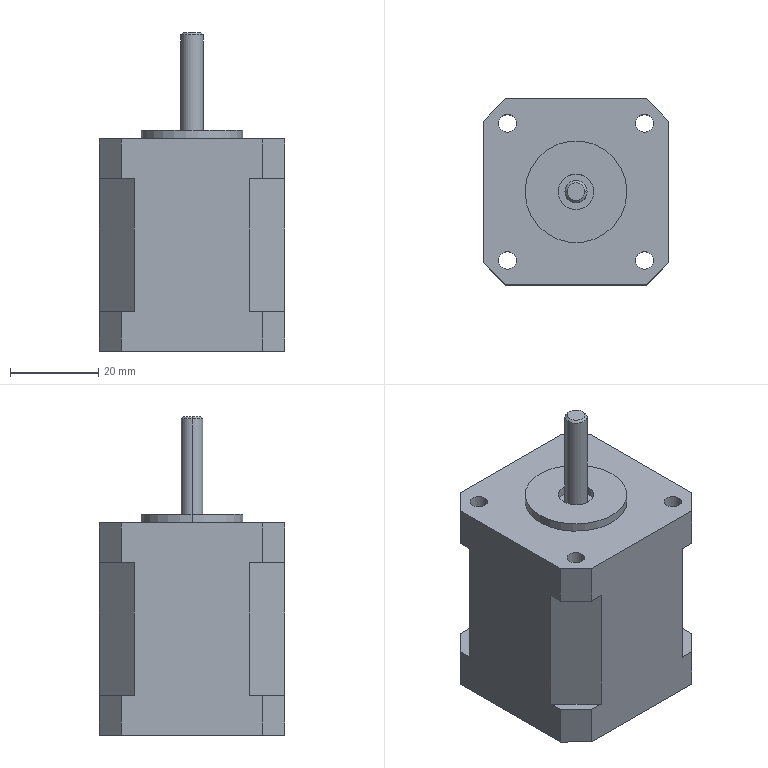Part | SolidWorks | features ICE 5, Chamfer 2, Extrusion 1, MirrorPattern 1 | 1 solid | 45 faces | box 42 x 42 x 72 mm | volume 78719 mm3 | plane 29 | cylinder 14 | cone 2 | commonest cylinder face diameters 4 x8 5 x2 8 x2 23 x2
STEP:
#1=CARTESIAN_POINT('',(-17.5,15.5,-24.));
#2=VERTEX_POINT('',#1);
#3=CARTESIAN_POINT('',(-13.5,15.5,-24.));
#4=VERTEX_POINT('',#3);
#5=CARTESIAN_POINT('',(-15.5,15.5,-24.));
#6=DIRECTION('',(0.,0.,1.));
#7=DIRECTION('',(1.,0.,0.));
#8=AXIS2_PLACEMENT_3D('',#5,#6,#7);
#9=CIRCLE('',#8,2.);
#10=EDGE_CURVE('',#2,#4,#9,.T.);
#11=ORIENTED_EDGE('',*,*,#10,.F.);
#12=CARTESIAN_POINT('',(-17.5,15.5,24.));
#13=VERTEX_POINT('',#12);
#14=CARTESIAN_POINT('',(-17.5,15.5,-24.));
#15=DIRECTION('',(0.,0.,1.));
#16=VECTOR('',#15,1000.);
#17=LINE('',#14,#16);
#18=EDGE_CURVE('',#2,#13,#17,.T.);
#19=ORIENTED_EDGE('',*,*,#18,.T.);
#20=CARTESIAN_POINT('',(-13.5,15.5,24.));
#21=VERTEX_POINT('',#20);
#22=CARTESIAN_POINT('',(-15.5,15.5,24.));
#23=DIRECTION('',(0.,0.,1.));
#24=DIRECTION('',(1.,0.,0.));
#25=AXIS2_PLACEMENT_3D('',#22,#23,#24);
#26=CIRCLE('',#25,2.);
#27=EDGE_CURVE('',#13,#21,#26,.T.);
#28=ORIENTED_EDGE('',*,*,#27,.T.);
#29=CARTESIAN_POINT('',(-13.5,15.5,-24.));
#30=DIRECTION('',(0.,0.,1.));
#31=VECTOR('',#30,1000.);
#32=LINE('',#29,#31);
#33=EDGE_CURVE('',#4,#21,#32,.T.);
#34=ORIENTED_EDGE('',*,*,#33,.F.);
#35=EDGE_LOOP('',(#11,#19,#28,#34));
#36=FACE_OUTER_BOUND('',#35,.T.);
#37=CARTESIAN_POINT('',(-15.5,15.5,-24.));
#38=DIRECTION('',(0.,0.,1.));
#39=DIRECTION('',(1.,0.,0.));
#40=AXIS2_PLACEMENT_3D('',#37,#38,#39);
#41=CYLINDRICAL_SURFACE('',#40,2.);
#42=ADVANCED_FACE('',(#36),#41,.F.);
#43=CARTESIAN_POINT('',(-17.5,-15.5,-24.));
#44=VERTEX_POINT('',#43);
#45=CARTESIAN_POINT('',(-13.5,-15.5,-24.));
#46=VERTEX_POINT('',#45);
#47=CARTESIAN_POINT('',(-15.5,-15.5,-24.));
#48=DIRECTION('',(0.,0.,1.));
#49=DIRECTION('',(1.,0.,0.));
#50=AXIS2_PLACEMENT_3D('',#47,#48,#49);
#51=CIRCLE('',#50,2.);
#52=EDGE_CURVE('',#44,#46,#51,.T.);
#53=ORIENTED_EDGE('',*,*,#52,.F.);
#54=CARTESIAN_POINT('',(-17.5,-15.5,24.));
#55=VERTEX_POINT('',#54);
#56=CARTESIAN_POINT('',(-17.5,-15.5,-24.));
#57=DIRECTION('',(0.,0.,1.));
#58=VECTOR('',#57,1000.);
#59=LINE('',#56,#58);
#60=EDGE_CURVE('',#44,#55,#59,.T.);
#61=ORIENTED_EDGE('',*,*,#60,.T.);
#62=CARTESIAN_POINT('',(-13.5,-15.5,24.));
#63=VERTEX_POINT('',#62);
#64=CARTESIAN_POINT('',(-15.5,-15.5,24.));
#65=DIRECTION('',(0.,0.,1.));
#66=DIRECTION('',(1.,0.,0.));
#67=AXIS2_PLACEMENT_3D('',#64,#65,#66);
#68=CIRCLE('',#67,2.);
#69=EDGE_CURVE('',#55,#63,#68,.T.);
#70=ORIENTED_EDGE('',*,*,#69,.T.);
#71=CARTESIAN_POINT('',(-13.5,-15.5,-24.));
#72=DIRECTION('',(0.,0.,1.));
#73=VECTOR('',#72,1000.);
#74=LINE('',#71,#73);
#75=EDGE_CURVE('',#46,#63,#74,.T.);
#76=ORIENTED_EDGE('',*,*,#75,.F.);
#77=EDGE_LOOP('',(#53,#61,#70,#76));
#78=FACE_OUTER_BOUND('',#77,.T.);
#79=CARTESIAN_POINT('',(-15.5,-15.5,-24.));
#80=DIRECTION('',(0.,0.,1.));
#81=DIRECTION('',(1.,0.,0.));
#82=AXIS2_PLACEMENT_3D('',#79,#80,#81);
#83=CYLINDRICAL_SURFACE('',#82,2.);
#84=ADVANCED_FACE('',(#78),#83,.F.);
#85=CARTESIAN_POINT('',(13.5,-15.5,-24.));
#86=VERTEX_POINT('',#85);
#87=CARTESIAN_POINT('',(17.5,-15.5,-24.));
#88=VERTEX_POINT('',#87);
#89=CARTESIAN_POINT('',(15.5,-15.5,-24.));
#90=DIRECTION('',(0.,0.,1.));
#91=DIRECTION('',(1.,0.,0.));
#92=AXIS2_PLACEMENT_3D('',#89,#90,#91);
#93=CIRCLE('',#92,2.);
#94=EDGE_CURVE('',#86,#88,#93,.T.);
#95=ORIENTED_EDGE('',*,*,#94,.F.);
#96=CARTESIAN_POINT('',(13.5,-15.5,24.));
#97=VERTEX_POINT('',#96);
#98=CARTESIAN_POINT('',(13.5,-15.5,-24.));
#99=DIRECTION('',(0.,0.,1.));
#100=VECTOR('',#99,1000.);
#101=LINE('',#98,#100);
#102=EDGE_CURVE('',#86,#97,#101,.T.);
#103=ORIENTED_EDGE('',*,*,#102,.T.);
#104=CARTESIAN_POINT('',(17.5,-15.5,24.));
#105=VERTEX_POINT('',#104);
#106=CARTESIAN_POINT('',(15.5,-15.5,24.));
#107=DIRECTION('',(0.,0.,1.));
#108=DIRECTION('',(1.,0.,0.));
#109=AXIS2_PLACEMENT_3D('',#106,#107,#108);
#110=CIRCLE('',#109,2.);
#111=EDGE_CURVE('',#97,#105,#110,.T.);
#112=ORIENTED_EDGE('',*,*,#111,.T.);
#113=CARTESIAN_POINT('',(17.5,-15.5,-24.));
#114=DIRECTION('',(0.,0.,1.));
#115=VECTOR('',#114,1000.);
#116=LINE('',#113,#115);
#117=EDGE_CURVE('',#88,#105,#116,.T.);
#118=ORIENTED_EDGE('',*,*,#117,.F.);
#119=EDGE_LOOP('',(#95,#103,#112,#118));
#120=FACE_OUTER_BOUND('',#119,.T.);
#121=CARTESIAN_POINT('',(15.5,-15.5,-24.));
#122=DIRECTION('',(0.,0.,1.));
#123=DIRECTION('',(1.,0.,0.));
#124=AXIS2_PLACEMENT_3D('',#121,#122,#123);
#125=CYLINDRICAL_SURFACE('',#124,2.);
#126=ADVANCED_FACE('',(#120),#125,.F.);
#127=CARTESIAN_POINT('',(13.5,15.5,-24.));
#128=VERTEX_POINT('',#127);
#129=CARTESIAN_POINT('',(17.5,15.5,-24.));
#130=VERTEX_POINT('',#129);
#131=CARTESIAN_POINT('',(15.5,15.5,-24.));
#132=DIRECTION('',(0.,0.,1.));
#133=DIRECTION('',(1.,0.,0.));
#134=AXIS2_PLACEMENT_3D('',#131,#132,#133);
#135=CIRCLE('',#134,2.);
#136=EDGE_CURVE('',#128,#130,#135,.T.);
#137=ORIENTED_EDGE('',*,*,#136,.F.);
#138=CARTESIAN_POINT('',(13.5,15.5,24.));
#139=VERTEX_POINT('',#138);
#140=CARTESIAN_POINT('',(13.5,15.5,-24.));
#141=DIRECTION('',(0.,0.,1.));
#142=VECTOR('',#141,1000.);
#143=LINE('',#140,#142);
#144=EDGE_CURVE('',#128,#139,#143,.T.);
#145=ORIENTED_EDGE('',*,*,#144,.T.);
#146=CARTESIAN_POINT('',(17.5,15.5,24.));
#147=VERTEX_POINT('',#146);
#148=CARTESIAN_POINT('',(15.5,15.5,24.));
#149=DIRECTION('',(0.,0.,1.));
#150=DIRECTION('',(1.,0.,0.));
#151=AXIS2_PLACEMENT_3D('',#148,#149,#150);
#152=CIRCLE('',#151,2.);
#153=EDGE_CURVE('',#139,#147,#152,.T.);
#154=ORIENTED_EDGE('',*,*,#153,.T.);
#155=CARTESIAN_POINT('',(17.5,15.5,-24.));
#156=DIRECTION('',(0.,0.,1.));
#157=VECTOR('',#156,1000.);
#158=LINE('',#155,#157);
#159=EDGE_CURVE('',#130,#147,#158,.T.);
#160=ORIENTED_EDGE('',*,*,#159,.F.);
#161=EDGE_LOOP('',(#137,#145,#154,#160));
#162=FACE_OUTER_BOUND('',#161,.T.);
#163=CARTESIAN_POINT('',(15.5,15.5,-24.));
#164=DIRECTION('',(0.,0.,1.));
#165=DIRECTION('',(1.,0.,0.));
#166=AXIS2_PLACEMENT_3D('',#163,#164,#165);
#167=CYLINDRICAL_SURFACE('',#166,2.);
#168=ADVANCED_FACE('',(#162),#167,.F.);
#169=CARTESIAN_POINT('',(2.,0.,48.));
#170=VERTEX_POINT('',#169);
#171=CARTESIAN_POINT('',(-2.,0.,48.));
#172=VERTEX_POINT('',#171);
#173=CARTESIAN_POINT('',(0.,0.,48.));
#174=DIRECTION('',(0.,0.,1.));
#175=DIRECTION('',(1.,0.,0.));
#176=AXIS2_PLACEMENT_3D('',#173,#174,#175);
#177=CIRCLE('',#176,2.);
#178=EDGE_CURVE('',#170,#172,#177,.T.);
#179=ORIENTED_EDGE('',*,*,#178,.F.);
#180=CARTESIAN_POINT('',(2.5,0.,47.5));
#181=VERTEX_POINT('',#180);
#182=CARTESIAN_POINT('',(2.,0.,48.));
#183=DIRECTION('',(0.7071,0.,-0.7071));
#184=VECTOR('',#183,1000.);
#185=LINE('',#182,#184);
#186=EDGE_CURVE('',#170,#181,#185,.T.);
#187=ORIENTED_EDGE('',*,*,#186,.T.);
#188=CARTESIAN_POINT('',(-2.5,0.,47.5));
#189=VERTEX_POINT('',#188);
#190=CARTESIAN_POINT('',(0.,0.,47.5));
#191=DIRECTION('',(0.,0.,-1.));
#192=DIRECTION('',(1.,0.,0.));
#193=AXIS2_PLACEMENT_3D('',#190,#191,#192);
#194=CIRCLE('',#193,2.5);
#195=EDGE_CURVE('',#189,#181,#194,.T.);
#196=ORIENTED_EDGE('',*,*,#195,.F.);
#197=CARTESIAN_POINT('',(-2.,0.,48.));
#198=DIRECTION('',(-0.7071,0.,-0.7071));
#199=VECTOR('',#198,1000.);
#200=LINE('',#197,#199);
#201=EDGE_CURVE('',#172,#189,#200,.T.);
#202=ORIENTED_EDGE('',*,*,#201,.F.);
#203=EDGE_LOOP('',(#179,#187,#196,#202));
#204=FACE_OUTER_BOUND('',#203,.T.);
#205=CARTESIAN_POINT('',(0.,0.,48.));
#206=DIRECTION('',(0.,0.,-1.));
#207=DIRECTION('',(-1.,0.,0.));
#208=AXIS2_PLACEMENT_3D('',#205,#206,#207);
#209=CONICAL_SURFACE('',#208,2.,0.7854);
#210=ADVANCED_FACE('',(#204),#209,.T.);
#211=ORIENTED_EDGE('',*,*,#195,.T.);
#212=CARTESIAN_POINT('',(2.5,0.,24.));
#213=VERTEX_POINT('',#212);
#214=CARTESIAN_POINT('',(2.5,0.,48.));
#215=DIRECTION('',(0.,0.,-1.));
#216=VECTOR('',#215,1000.);
#217=LINE('',#214,#216);
#218=EDGE_CURVE('',#181,#213,#217,.T.);
#219=ORIENTED_EDGE('',*,*,#218,.T.);
#220=CARTESIAN_POINT('',(-2.5,0.,24.));
#221=VERTEX_POINT('',#220);
#222=CARTESIAN_POINT('',(0.,0.,24.));
#223=DIRECTION('',(0.,0.,1.));
#224=DIRECTION('',(1.,0.,0.));
#225=AXIS2_PLACEMENT_3D('',#222,#223,#224);
#226=CIRCLE('',#225,2.5);
#227=EDGE_CURVE('',#213,#221,#226,.T.);
#228=ORIENTED_EDGE('',*,*,#227,.T.);
#229=CARTESIAN_POINT('',(-2.5,0.,48.));
#230=DIRECTION('',(0.,0.,-1.));
#231=VECTOR('',#230,1000.);
#232=LINE('',#229,#231);
#233=EDGE_CURVE('',#189,#221,#232,.T.);
#234=ORIENTED_EDGE('',*,*,#233,.F.);
#235=EDGE_LOOP('',(#211,#219,#228,#234));
#236=FACE_OUTER_BOUND('',#235,.T.);
#237=CARTESIAN_POINT('',(0.,0.,48.));
#238=DIRECTION('',(0.,0.,-1.));
#239=DIRECTION('',(-1.,0.,0.));
#240=AXIS2_PLACEMENT_3D('',#237,#238,#239);
#241=CYLINDRICAL_SURFACE('',#240,2.5);
#242=ADVANCED_FACE('',(#236),#241,.T.);
#243=CARTESIAN_POINT('',(-4.,0.,24.));
#244=VERTEX_POINT('',#243);
#245=CARTESIAN_POINT('',(4.,0.,24.));
#246=VERTEX_POINT('',#245);
#247=CARTESIAN_POINT('',(0.,0.,24.));
#248=DIRECTION('',(0.,0.,1.));
#249=DIRECTION('',(1.,0.,0.));
#250=AXIS2_PLACEMENT_3D('',#247,#248,#249);
#251=CIRCLE('',#250,4.);
#252=EDGE_CURVE('',#244,#246,#251,.T.);
#253=ORIENTED_EDGE('',*,*,#252,.F.);
#254=CARTESIAN_POINT('',(-4.,0.,26.));
#255=VERTEX_POINT('',#254);
#256=CARTESIAN_POINT('',(-4.,0.,24.));
#257=DIRECTION('',(0.,0.,1.));
#258=VECTOR('',#257,1000.);
#259=LINE('',#256,#258);
#260=EDGE_CURVE('',#244,#255,#259,.T.);
#261=ORIENTED_EDGE('',*,*,#260,.T.);
#262=CARTESIAN_POINT('',(4.,0.,26.));
#263=VERTEX_POINT('',#262);
#264=CARTESIAN_POINT('',(0.,0.,26.));
#265=DIRECTION('',(0.,0.,1.));
#266=DIRECTION('',(1.,0.,0.));
#267=AXIS2_PLACEMENT_3D('',#264,#265,#266);
#268=CIRCLE('',#267,4.);
#269=EDGE_CURVE('',#255,#263,#268,.T.);
#270=ORIENTED_EDGE('',*,*,#269,.T.);
#271=CARTESIAN_POINT('',(4.,0.,24.));
#272=DIRECTION('',(0.,0.,1.));
#273=VECTOR('',#272,1000.);
#274=LINE('',#271,#273);
#275=EDGE_CURVE('',#246,#263,#274,.T.);
#276=ORIENTED_EDGE('',*,*,#275,.F.);
#277=EDGE_LOOP('',(#253,#261,#270,#276));
#278=FACE_OUTER_BOUND('',#277,.T.);
#279=CARTESIAN_POINT('',(0.,0.,24.));
#280=DIRECTION('',(0.,0.,1.));
#281=DIRECTION('',(1.,0.,0.));
#282=AXIS2_PLACEMENT_3D('',#279,#280,#281);
#283=CYLINDRICAL_SURFACE('',#282,4.);
#284=ADVANCED_FACE('',(#278),#283,.F.);
#285=CARTESIAN_POINT('',(11.5,0.,26.));
#286=VERTEX_POINT('',#285);
#287=CARTESIAN_POINT('',(-11.5,0.,26.));
#288=VERTEX_POINT('',#287);
#289=CARTESIAN_POINT('',(0.,0.,26.));
#290=DIRECTION('',(0.,0.,1.));
#291=DIRECTION('',(1.,0.,0.));
#292=AXIS2_PLACEMENT_3D('',#289,#290,#291);
#293=CIRCLE('',#292,11.5);
#294=EDGE_CURVE('',#286,#288,#293,.T.);
#295=ORIENTED_EDGE('',*,*,#294,.F.);
#296=CARTESIAN_POINT('',(11.5,0.,24.));
#297=VERTEX_POINT('',#296);
#298=CARTESIAN_POINT('',(11.5,0.,26.));
#299=DIRECTION('',(0.,0.,-1.));
#300=VECTOR('',#299,1000.);
#301=LINE('',#298,#300);
#302=EDGE_CURVE('',#286,#297,#301,.T.);
#303=ORIENTED_EDGE('',*,*,#302,.T.);
#304=CARTESIAN_POINT('',(-11.5,0.,24.));
#305=VERTEX_POINT('',#304);
#306=CARTESIAN_POINT('',(0.,0.,24.));
#307=DIRECTION('',(0.,0.,1.));
#308=DIRECTION('',(-1.,0.,0.));
#309=AXIS2_PLACEMENT_3D('',#306,#307,#308);
#310=CIRCLE('',#309,11.5);
#311=EDGE_CURVE('',#297,#305,#310,.T.);
#312=ORIENTED_EDGE('',*,*,#311,.T.);
#313=CARTESIAN_POINT('',(-11.5,0.,26.));
#314=DIRECTION('',(0.,0.,-1.));
#315=VECTOR('',#314,1000.);
#316=LINE('',#313,#315);
#317=EDGE_CURVE('',#288,#305,#316,.T.);
#318=ORIENTED_EDGE('',*,*,#317,.F.);
#319=EDGE_LOOP('',(#295,#303,#312,#318));
#320=FACE_OUTER_BOUND('',#319,.T.);
#321=CARTESIAN_POINT('',(0.,0.,26.));
#322=DIRECTION('',(0.,0.,-1.));
#323=DIRECTION('',(-1.,0.,0.));
#324=AXIS2_PLACEMENT_3D('',#321,#322,#323);
#325=CYLINDRICAL_SURFACE('',#324,11.5);
#326=ADVANCED_FACE('',(#320),#325,.T.);
#327=CARTESIAN_POINT('',(0.,0.,26.));
#328=DIRECTION('',(0.,0.,1.));
#329=DIRECTION('',(1.,0.,0.));
#330=AXIS2_PLACEMENT_3D('',#327,#328,#329);
#331=CIRCLE('',#330,4.);
#332=EDGE_CURVE('',#263,#255,#331,.T.);
#333=ORIENTED_EDGE('',*,*,#332,.F.);
#334=ORIENTED_EDGE('',*,*,#269,.F.);
#335=EDGE_LOOP('',(#333,#334));
#336=FACE_BOUND('',#335,.T.);
#337=CARTESIAN_POINT('',(0.,0.,26.));
#338=DIRECTION('',(0.,0.,1.));
#339=DIRECTION('',(1.,0.,0.));
#340=AXIS2_PLACEMENT_3D('',#337,#338,#339);
#341=CIRCLE('',#340,11.5);
#342=EDGE_CURVE('',#288,#286,#341,.T.);
#343=ORIENTED_EDGE('',*,*,#342,.T.);
#344=ORIENTED_EDGE('',*,*,#294,.T.);
#345=EDGE_LOOP('',(#343,#344));
#346=FACE_OUTER_BOUND('',#345,.T.);
#347=CARTESIAN_POINT('',(0.,0.,26.));
#348=DIRECTION('',(0.,0.,1.));
#349=DIRECTION('',(1.,0.,0.));
#350=AXIS2_PLACEMENT_3D('',#347,#348,#349);
#351=PLANE('',#350);
#352=ADVANCED_FACE('',(#336,#346),#351,.T.);
#353=CARTESIAN_POINT('',(-15.5,15.5,24.));
#354=DIRECTION('',(0.,0.,1.));
#355=DIRECTION('',(1.,0.,0.));
#356=AXIS2_PLACEMENT_3D('',#353,#354,#355);
#357=CIRCLE('',#356,2.);
#358=EDGE_CURVE('',#21,#13,#357,.T.);
#359=ORIENTED_EDGE('',*,*,#358,.F.);
#360=ORIENTED_EDGE('',*,*,#27,.F.);
#361=EDGE_LOOP('',(#359,#360));
#362=FACE_BOUND('',#361,.T.);
#363=CARTESIAN_POINT('',(-15.5,-15.5,24.));
#364=DIRECTION('',(0.,0.,1.));
#365=DIRECTION('',(1.,0.,0.));
#366=AXIS2_PLACEMENT_3D('',#363,#364,#365);
#367=CIRCLE('',#366,2.);
#368=EDGE_CURVE('',#63,#55,#367,.T.);
#369=ORIENTED_EDGE('',*,*,#368,.F.);
#370=ORIENTED_EDGE('',*,*,#69,.F.);
#371=EDGE_LOOP('',(#369,#370));
#372=FACE_BOUND('',#371,.T.);
#373=CARTESIAN_POINT('',(15.5,-15.5,24.));
#374=DIRECTION('',(0.,0.,1.));
#375=DIRECTION('',(1.,0.,0.));
#376=AXIS2_PLACEMENT_3D('',#373,#374,#375);
#377=CIRCLE('',#376,2.);
#378=EDGE_CURVE('',#105,#97,#377,.T.);
#379=ORIENTED_EDGE('',*,*,#378,.F.);
#380=ORIENTED_EDGE('',*,*,#111,.F.);
#381=EDGE_LOOP('',(#379,#380));
#382=FACE_BOUND('',#381,.T.);
#383=CARTESIAN_POINT('',(15.5,15.5,24.));
#384=DIRECTION('',(0.,0.,1.));
#385=DIRECTION('',(1.,0.,0.));
#386=AXIS2_PLACEMENT_3D('',#383,#384,#385);
#387=CIRCLE('',#386,2.);
#388=EDGE_CURVE('',#147,#139,#387,.T.);
#389=ORIENTED_EDGE('',*,*,#388,.F.);
#390=ORIENTED_EDGE('',*,*,#153,.F.);
#391=EDGE_LOOP('',(#389,#390));
#392=FACE_BOUND('',#391,.T.);
#393=CARTESIAN_POINT('',(-16.,21.,24.));
#394=VERTEX_POINT('',#393);
#395=CARTESIAN_POINT('',(-21.,16.,24.));
#396=VERTEX_POINT('',#395);
#397=CARTESIAN_POINT('',(-16.,21.,24.));
#398=DIRECTION('',(-0.7071,-0.7071,0.));
#399=VECTOR('',#398,1000.);
#400=LINE('',#397,#399);
#401=EDGE_CURVE('',#394,#396,#400,.T.);
#402=ORIENTED_EDGE('',*,*,#401,.T.);
#403=CARTESIAN_POINT('',(-21.,-16.,24.));
#404=VERTEX_POINT('',#403);
#405=CARTESIAN_POINT('',(-21.,-16.,24.));
#406=DIRECTION('',(0.,-1.,0.));
#407=VECTOR('',#406,1000.);
#408=LINE('',#405,#407);
#409=EDGE_CURVE('',#396,#404,#408,.T.);
#410=ORIENTED_EDGE('',*,*,#409,.T.);
#411=CARTESIAN_POINT('',(-16.,-21.,24.));
#412=VERTEX_POINT('',#411);
#413=CARTESIAN_POINT('',(-16.,-21.,24.));
#414=DIRECTION('',(0.7071,-0.7071,0.));
#415=VECTOR('',#414,1000.);
#416=LINE('',#413,#415);
#417=EDGE_CURVE('',#404,#412,#416,.T.);
#418=ORIENTED_EDGE('',*,*,#417,.T.);
#419=CARTESIAN_POINT('',(16.,-21.,24.));
#420=VERTEX_POINT('',#419);
#421=CARTESIAN_POINT('',(16.,-21.,24.));
#422=DIRECTION('',(1.,0.,0.));
#423=VECTOR('',#422,1000.);
#424=LINE('',#421,#423);
#425=EDGE_CURVE('',#412,#420,#424,.T.);
#426=ORIENTED_EDGE('',*,*,#425,.T.);
#427=CARTESIAN_POINT('',(21.,-16.,24.));
#428=VERTEX_POINT('',#427);
#429=CARTESIAN_POINT('',(21.,-16.,24.));
#430=DIRECTION('',(0.7071,0.7071,0.));
#431=VECTOR('',#430,1000.);
#432=LINE('',#429,#431);
#433=EDGE_CURVE('',#420,#428,#432,.T.);
#434=ORIENTED_EDGE('',*,*,#433,.T.);
#435=CARTESIAN_POINT('',(21.,16.,24.));
#436=VERTEX_POINT('',#435);
#437=CARTESIAN_POINT('',(21.,-16.,24.));
#438=DIRECTION('',(0.,1.,0.));
#439=VECTOR('',#438,1000.);
#440=LINE('',#437,#439);
#441=EDGE_CURVE('',#428,#436,#440,.T.);
#442=ORIENTED_EDGE('',*,*,#441,.T.);
#443=CARTESIAN_POINT('',(16.,21.,24.));
#444=VERTEX_POINT('',#443);
#445=CARTESIAN_POINT('',(21.,16.,24.));
#446=DIRECTION('',(-0.7071,0.7071,0.));
#447=VECTOR('',#446,1000.);
#448=LINE('',#445,#447);
#449=EDGE_CURVE('',#436,#444,#448,.T.);
#450=ORIENTED_EDGE('',*,*,#449,.T.);
#451=CARTESIAN_POINT('',(16.,21.,24.));
#452=DIRECTION('',(-1.,0.,0.));
#453=VECTOR('',#452,1000.);
#454=LINE('',#451,#453);
#455=EDGE_CURVE('',#444,#394,#454,.T.);
#456=ORIENTED_EDGE('',*,*,#455,.T.);
#457=EDGE_LOOP('',(#402,#410,#418,#426,#434,#442,#450,#456));
#458=FACE_OUTER_BOUND('',#457,.T.);
#459=CARTESIAN_POINT('',(0.,0.,24.));
#460=DIRECTION('',(0.,0.,1.));
#461=DIRECTION('',(-1.,0.,0.));
#462=AXIS2_PLACEMENT_3D('',#459,#460,#461);
#463=CIRCLE('',#462,11.5);
#464=EDGE_CURVE('',#305,#297,#463,.T.);
#465=ORIENTED_EDGE('',*,*,#464,.F.);
#466=ORIENTED_EDGE('',*,*,#311,.F.);
#467=EDGE_LOOP('',(#465,#466));
#468=FACE_BOUND('',#467,.T.);
#469=CARTESIAN_POINT('',(0.,0.,24.));
#470=DIRECTION('',(0.,0.,-1.));
#471=DIRECTION('',(-1.,0.,0.));
#472=AXIS2_PLACEMENT_3D('',#469,#470,#471);
#473=PLANE('',#472);
#474=ADVANCED_FACE('',(#362,#372,#382,#392,#458,#468),#473,.F.);
#475=CARTESIAN_POINT('',(-21.,13.,15.));
#476=VERTEX_POINT('',#475);
#477=CARTESIAN_POINT('',(-21.,13.,-15.));
#478=VERTEX_POINT('',#477);
#479=CARTESIAN_POINT('',(-21.,13.,15.));
#480=DIRECTION('',(0.,0.,-1.));
#481=VECTOR('',#480,1000.);
#482=LINE('',#479,#481);
#483=EDGE_CURVE('',#476,#478,#482,.T.);
#484=ORIENTED_EDGE('',*,*,#483,.T.);
#485=CARTESIAN_POINT('',(-21.,16.,-15.));
#486=VERTEX_POINT('',#485);
#487=CARTESIAN_POINT('',(-21.,-16.,-15.));
#488=DIRECTION('',(0.,-1.,0.));
#489=VECTOR('',#488,1000.);
#490=LINE('',#487,#489);
#491=EDGE_CURVE('',#486,#478,#490,.T.);
#492=ORIENTED_EDGE('',*,*,#491,.F.);
#493=CARTESIAN_POINT('',(-21.,16.,-24.));
#494=VERTEX_POINT('',#493);
#495=CARTESIAN_POINT('',(-21.,16.,-24.));
#496=DIRECTION('',(0.,0.,1.));
#497=VECTOR('',#496,1000.);
#498=LINE('',#495,#497);
#499=EDGE_CURVE('',#494,#486,#498,.T.);
#500=ORIENTED_EDGE('',*,*,#499,.F.);
#501=CARTESIAN_POINT('',(-21.,-16.,-24.));
#502=VERTEX_POINT('',#501);
#503=CARTESIAN_POINT('',(-21.,-16.,-24.));
#504=DIRECTION('',(0.,-1.,0.));
#505=VECTOR('',#504,1000.);
#506=LINE('',#503,#505);
#507=EDGE_CURVE('',#494,#502,#506,.T.);
#508=ORIENTED_EDGE('',*,*,#507,.T.);
#509=CARTESIAN_POINT('',(-21.,-16.,-15.));
#510=VERTEX_POINT('',#509);
#511=CARTESIAN_POINT('',(-21.,-16.,-24.));
#512=DIRECTION('',(0.,0.,1.));
#513=VECTOR('',#512,1000.);
#514=LINE('',#511,#513);
#515=EDGE_CURVE('',#502,#510,#514,.T.);
#516=ORIENTED_EDGE('',*,*,#515,.T.);
#517=CARTESIAN_POINT('',(-21.,-13.,-15.));
#518=VERTEX_POINT('',#517);
#519=CARTESIAN_POINT('',(-21.,-16.,-15.));
#520=DIRECTION('',(0.,-1.,0.));
#521=VECTOR('',#520,1000.);
#522=LINE('',#519,#521);
#523=EDGE_CURVE('',#518,#510,#522,.T.);
#524=ORIENTED_EDGE('',*,*,#523,.F.);
#525=CARTESIAN_POINT('',(-21.,-13.,15.));
#526=VERTEX_POINT('',#525);
#527=CARTESIAN_POINT('',(-21.,-13.,15.));
#528=DIRECTION('',(0.,0.,1.));
#529=VECTOR('',#528,1000.);
#530=LINE('',#527,#529);
#531=EDGE_CURVE('',#518,#526,#530,.T.);
#532=ORIENTED_EDGE('',*,*,#531,.T.);
#533=CARTESIAN_POINT('',(-21.,-16.,15.));
#534=VERTEX_POINT('',#533);
#535=CARTESIAN_POINT('',(-21.,-16.,15.));
#536=DIRECTION('',(0.,-1.,0.));
#537=VECTOR('',#536,1000.);
#538=LINE('',#535,#537);
#539=EDGE_CURVE('',#526,#534,#538,.T.);
#540=ORIENTED_EDGE('',*,*,#539,.T.);
#541=CARTESIAN_POINT('',(-21.,-16.,24.));
#542=DIRECTION('',(0.,0.,-1.));
#543=VECTOR('',#542,1000.);
#544=LINE('',#541,#543);
#545=EDGE_CURVE('',#404,#534,#544,.T.);
#546=ORIENTED_EDGE('',*,*,#545,.F.);
#547=ORIENTED_EDGE('',*,*,#409,.F.);
#548=CARTESIAN_POINT('',(-21.,16.,15.));
#549=VERTEX_POINT('',#548);
#550=CARTESIAN_POINT('',(-21.,16.,24.));
#551=DIRECTION('',(0.,0.,-1.));
#552=VECTOR('',#551,1000.);
#553=LINE('',#550,#552);
#554=EDGE_CURVE('',#396,#549,#553,.T.);
#555=ORIENTED_EDGE('',*,*,#554,.T.);
#556=CARTESIAN_POINT('',(-21.,-16.,15.));
#557=DIRECTION('',(0.,-1.,0.));
#558=VECTOR('',#557,1000.);
#559=LINE('',#556,#558);
#560=EDGE_CURVE('',#549,#476,#559,.T.);
#561=ORIENTED_EDGE('',*,*,#560,.T.);
#562=EDGE_LOOP('',(#484,#492,#500,#508,#516,#524,#532,#540,#546,#547,#555,#561));
#563=FACE_OUTER_BOUND('',#562,.T.);
#564=CARTESIAN_POINT('',(-21.,-21.,15.));
#565=DIRECTION('',(1.,0.,0.));
#566=DIRECTION('',(0.,0.,-1.));
#567=AXIS2_PLACEMENT_3D('',#564,#565,#566);
#568=PLANE('',#567);
#569=ADVANCED_FACE('',(#563),#568,.F.);
#570=CARTESIAN_POINT('',(13.,-21.,-15.));
#571=VERTEX_POINT('',#570);
#572=CARTESIAN_POINT('',(13.,-21.,15.));
#573=VERTEX_POINT('',#572);
#574=CARTESIAN_POINT('',(13.,-21.,15.));
#575=DIRECTION('',(0.,0.,1.));
#576=VECTOR('',#575,1000.);
#577=LINE('',#574,#576);
#578=EDGE_CURVE('',#571,#573,#577,.T.);
#579=ORIENTED_EDGE('',*,*,#578,.T.);
#580=CARTESIAN_POINT('',(16.,-21.,15.));
#581=VERTEX_POINT('',#580);
#582=CARTESIAN_POINT('',(16.,-21.,15.));
#583=DIRECTION('',(1.,0.,0.));
#584=VECTOR('',#583,1000.);
#585=LINE('',#582,#584);
#586=EDGE_CURVE('',#573,#581,#585,.T.);
#587=ORIENTED_EDGE('',*,*,#586,.T.);
#588=CARTESIAN_POINT('',(16.,-21.,24.));
#589=DIRECTION('',(0.,0.,-1.));
#590=VECTOR('',#589,1000.);
#591=LINE('',#588,#590);
#592=EDGE_CURVE('',#420,#581,#591,.T.);
#593=ORIENTED_EDGE('',*,*,#592,.F.);
#594=ORIENTED_EDGE('',*,*,#425,.F.);
#595=CARTESIAN_POINT('',(-16.,-21.,15.));
#596=VERTEX_POINT('',#595);
#597=CARTESIAN_POINT('',(-16.,-21.,24.));
#598=DIRECTION('',(0.,0.,-1.));
#599=VECTOR('',#598,1000.);
#600=LINE('',#597,#599);
#601=EDGE_CURVE('',#412,#596,#600,.T.);
#602=ORIENTED_EDGE('',*,*,#601,.T.);
#603=CARTESIAN_POINT('',(-13.,-21.,15.));
#604=VERTEX_POINT('',#603);
#605=CARTESIAN_POINT('',(16.,-21.,15.));
#606=DIRECTION('',(1.,0.,0.));
#607=VECTOR('',#606,1000.);
#608=LINE('',#605,#607);
#609=EDGE_CURVE('',#596,#604,#608,.T.);
#610=ORIENTED_EDGE('',*,*,#609,.T.);
#611=CARTESIAN_POINT('',(-13.,-21.,-15.));
#612=VERTEX_POINT('',#611);
#613=CARTESIAN_POINT('',(-13.,-21.,15.));
#614=DIRECTION('',(0.,0.,-1.));
#615=VECTOR('',#614,1000.);
#616=LINE('',#613,#615);
#617=EDGE_CURVE('',#604,#612,#616,.T.);
#618=ORIENTED_EDGE('',*,*,#617,.T.);
#619=CARTESIAN_POINT('',(-16.,-21.,-15.));
#620=VERTEX_POINT('',#619);
#621=CARTESIAN_POINT('',(16.,-21.,-15.));
#622=DIRECTION('',(1.,0.,0.));
#623=VECTOR('',#622,1000.);
#624=LINE('',#621,#623);
#625=EDGE_CURVE('',#620,#612,#624,.T.);
#626=ORIENTED_EDGE('',*,*,#625,.F.);
#627=CARTESIAN_POINT('',(-16.,-21.,-24.));
#628=VERTEX_POINT('',#627);
#629=CARTESIAN_POINT('',(-16.,-21.,-24.));
#630=DIRECTION('',(0.,0.,1.));
#631=VECTOR('',#630,1000.);
#632=LINE('',#629,#631);
#633=EDGE_CURVE('',#628,#620,#632,.T.);
#634=ORIENTED_EDGE('',*,*,#633,.F.);
#635=CARTESIAN_POINT('',(16.,-21.,-24.));
#636=VERTEX_POINT('',#635);
#637=CARTESIAN_POINT('',(16.,-21.,-24.));
#638=DIRECTION('',(1.,0.,0.));
#639=VECTOR('',#638,1000.);
#640=LINE('',#637,#639);
#641=EDGE_CURVE('',#628,#636,#640,.T.);
#642=ORIENTED_EDGE('',*,*,#641,.T.);
#643=CARTESIAN_POINT('',(16.,-21.,-15.));
#644=VERTEX_POINT('',#643);
#645=CARTESIAN_POINT('',(16.,-21.,-24.));
#646=DIRECTION('',(0.,0.,1.));
#647=VECTOR('',#646,1000.);
#648=LINE('',#645,#647);
#649=EDGE_CURVE('',#636,#644,#648,.T.);
#650=ORIENTED_EDGE('',*,*,#649,.T.);
#651=CARTESIAN_POINT('',(16.,-21.,-15.));
#652=DIRECTION('',(1.,0.,0.));
#653=VECTOR('',#652,1000.);
#654=LINE('',#651,#653);
#655=EDGE_CURVE('',#571,#644,#654,.T.);
#656=ORIENTED_EDGE('',*,*,#655,.F.);
#657=EDGE_LOOP('',(#579,#587,#593,#594,#602,#610,#618,#626,#634,#642,#650,#656));
#658=FACE_OUTER_BOUND('',#657,.T.);
#659=CARTESIAN_POINT('',(21.,-21.,15.));
#660=DIRECTION('',(0.,1.,0.));
#661=DIRECTION('',(-1.,0.,0.));
#662=AXIS2_PLACEMENT_3D('',#659,#660,#661);
#663=PLANE('',#662);
#664=ADVANCED_FACE('',(#658),#663,.F.);
#665=CARTESIAN_POINT('',(21.,13.,-15.));
#666=VERTEX_POINT('',#665);
#667=CARTESIAN_POINT('',(21.,13.,15.));
#668=VERTEX_POINT('',#667);
#669=CARTESIAN_POINT('',(21.,13.,15.));
#670=DIRECTION('',(0.,0.,1.));
#671=VECTOR('',#670,1000.);
#672=LINE('',#669,#671);
#673=EDGE_CURVE('',#666,#668,#672,.T.);
#674=ORIENTED_EDGE('',*,*,#673,.T.);
#675=CARTESIAN_POINT('',(21.,16.,15.));
#676=VERTEX_POINT('',#675);
#677=CARTESIAN_POINT('',(21.,-16.,15.));
#678=DIRECTION('',(0.,1.,0.));
#679=VECTOR('',#678,1000.);
#680=LINE('',#677,#679);
#681=EDGE_CURVE('',#668,#676,#680,.T.);
#682=ORIENTED_EDGE('',*,*,#681,.T.);
#683=CARTESIAN_POINT('',(21.,16.,24.));
#684=DIRECTION('',(0.,0.,-1.));
#685=VECTOR('',#684,1000.);
#686=LINE('',#683,#685);
#687=EDGE_CURVE('',#436,#676,#686,.T.);
#688=ORIENTED_EDGE('',*,*,#687,.F.);
#689=ORIENTED_EDGE('',*,*,#441,.F.);
#690=CARTESIAN_POINT('',(21.,-16.,15.));
#691=VERTEX_POINT('',#690);
#692=CARTESIAN_POINT('',(21.,-16.,24.));
#693=DIRECTION('',(0.,0.,-1.));
#694=VECTOR('',#693,1000.);
#695=LINE('',#692,#694);
#696=EDGE_CURVE('',#428,#691,#695,.T.);
#697=ORIENTED_EDGE('',*,*,#696,.T.);
#698=CARTESIAN_POINT('',(21.,-13.,15.));
#699=VERTEX_POINT('',#698);
#700=CARTESIAN_POINT('',(21.,-16.,15.));
#701=DIRECTION('',(0.,1.,0.));
#702=VECTOR('',#701,1000.);
#703=LINE('',#700,#702);
#704=EDGE_CURVE('',#691,#699,#703,.T.);
#705=ORIENTED_EDGE('',*,*,#704,.T.);
#706=CARTESIAN_POINT('',(21.,-13.,-15.));
#707=VERTEX_POINT('',#706);
#708=CARTESIAN_POINT('',(21.,-13.,15.));
#709=DIRECTION('',(0.,0.,-1.));
#710=VECTOR('',#709,1000.);
#711=LINE('',#708,#710);
#712=EDGE_CURVE('',#699,#707,#711,.T.);
#713=ORIENTED_EDGE('',*,*,#712,.T.);
#714=CARTESIAN_POINT('',(21.,-16.,-15.));
#715=VERTEX_POINT('',#714);
#716=CARTESIAN_POINT('',(21.,-16.,-15.));
#717=DIRECTION('',(0.,1.,0.));
#718=VECTOR('',#717,1000.);
#719=LINE('',#716,#718);
#720=EDGE_CURVE('',#715,#707,#719,.T.);
#721=ORIENTED_EDGE('',*,*,#720,.F.);
#722=CARTESIAN_POINT('',(21.,-16.,-24.));
#723=VERTEX_POINT('',#722);
#724=CARTESIAN_POINT('',(21.,-16.,-24.));
#725=DIRECTION('',(0.,0.,1.));
#726=VECTOR('',#725,1000.);
#727=LINE('',#724,#726);
#728=EDGE_CURVE('',#723,#715,#727,.T.);
#729=ORIENTED_EDGE('',*,*,#728,.F.);
#730=CARTESIAN_POINT('',(21.,16.,-24.));
#731=VERTEX_POINT('',#730);
#732=CARTESIAN_POINT('',(21.,-16.,-24.));
#733=DIRECTION('',(0.,1.,0.));
#734=VECTOR('',#733,1000.);
#735=LINE('',#732,#734);
#736=EDGE_CURVE('',#723,#731,#735,.T.);
#737=ORIENTED_EDGE('',*,*,#736,.T.);
#738=CARTESIAN_POINT('',(21.,16.,-15.));
#739=VERTEX_POINT('',#738);
#740=CARTESIAN_POINT('',(21.,16.,-24.));
#741=DIRECTION('',(0.,0.,1.));
#742=VECTOR('',#741,1000.);
#743=LINE('',#740,#742);
#744=EDGE_CURVE('',#731,#739,#743,.T.);
#745=ORIENTED_EDGE('',*,*,#744,.T.);
#746=CARTESIAN_POINT('',(21.,-16.,-15.));
#747=DIRECTION('',(0.,1.,0.));
#748=VECTOR('',#747,1000.);
#749=LINE('',#746,#748);
#750=EDGE_CURVE('',#666,#739,#749,.T.);
#751=ORIENTED_EDGE('',*,*,#750,.F.);
#752=EDGE_LOOP('',(#674,#682,#688,#689,#697,#705,#713,#721,#729,#737,#745,#751));
#753=FACE_OUTER_BOUND('',#752,.T.);
#754=CARTESIAN_POINT('',(21.,-21.,15.));
#755=DIRECTION('',(-1.,0.,0.));
#756=DIRECTION('',(0.,0.,1.));
#757=AXIS2_PLACEMENT_3D('',#754,#755,#756);
#758=PLANE('',#757);
#759=ADVANCED_FACE('',(#753),#758,.F.);
#760=CARTESIAN_POINT('',(13.,21.,15.));
#761=VERTEX_POINT('',#760);
#762=CARTESIAN_POINT('',(13.,21.,-15.));
#763=VERTEX_POINT('',#762);
#764=CARTESIAN_POINT('',(13.,21.,15.));
#765=DIRECTION('',(0.,0.,-1.));
#766=VECTOR('',#765,1000.);
#767=LINE('',#764,#766);
#768=EDGE_CURVE('',#761,#763,#767,.T.);
#769=ORIENTED_EDGE('',*,*,#768,.T.);
#770=CARTESIAN_POINT('',(16.,21.,-15.));
#771=VERTEX_POINT('',#770);
#772=CARTESIAN_POINT('',(16.,21.,-15.));
#773=DIRECTION('',(-1.,0.,0.));
#774=VECTOR('',#773,1000.);
#775=LINE('',#772,#774);
#776=EDGE_CURVE('',#771,#763,#775,.T.);
#777=ORIENTED_EDGE('',*,*,#776,.F.);
#778=CARTESIAN_POINT('',(16.,21.,-24.));
#779=VERTEX_POINT('',#778);
#780=CARTESIAN_POINT('',(16.,21.,-24.));
#781=DIRECTION('',(0.,0.,1.));
#782=VECTOR('',#781,1000.);
#783=LINE('',#780,#782);
#784=EDGE_CURVE('',#779,#771,#783,.T.);
#785=ORIENTED_EDGE('',*,*,#784,.F.);
#786=CARTESIAN_POINT('',(-16.,21.,-24.));
#787=VERTEX_POINT('',#786);
#788=CARTESIAN_POINT('',(16.,21.,-24.));
#789=DIRECTION('',(-1.,0.,0.));
#790=VECTOR('',#789,1000.);
#791=LINE('',#788,#790);
#792=EDGE_CURVE('',#779,#787,#791,.T.);
#793=ORIENTED_EDGE('',*,*,#792,.T.);
#794=CARTESIAN_POINT('',(-16.,21.,-15.));
#795=VERTEX_POINT('',#794);
#796=CARTESIAN_POINT('',(-16.,21.,-24.));
#797=DIRECTION('',(0.,0.,1.));
#798=VECTOR('',#797,1000.);
#799=LINE('',#796,#798);
#800=EDGE_CURVE('',#787,#795,#799,.T.);
#801=ORIENTED_EDGE('',*,*,#800,.T.);
#802=CARTESIAN_POINT('',(-13.,21.,-15.));
#803=VERTEX_POINT('',#802);
#804=CARTESIAN_POINT('',(16.,21.,-15.));
#805=DIRECTION('',(-1.,0.,0.));
#806=VECTOR('',#805,1000.);
#807=LINE('',#804,#806);
#808=EDGE_CURVE('',#803,#795,#807,.T.);
#809=ORIENTED_EDGE('',*,*,#808,.F.);
#810=CARTESIAN_POINT('',(-13.,21.,15.));
#811=VERTEX_POINT('',#810);
#812=CARTESIAN_POINT('',(-13.,21.,15.));
#813=DIRECTION('',(0.,0.,1.));
#814=VECTOR('',#813,1000.);
#815=LINE('',#812,#814);
#816=EDGE_CURVE('',#803,#811,#815,.T.);
#817=ORIENTED_EDGE('',*,*,#816,.T.);
#818=CARTESIAN_POINT('',(-16.,21.,15.));
#819=VERTEX_POINT('',#818);
#820=CARTESIAN_POINT('',(16.,21.,15.));
#821=DIRECTION('',(-1.,0.,0.));
#822=VECTOR('',#821,1000.);
#823=LINE('',#820,#822);
#824=EDGE_CURVE('',#811,#819,#823,.T.);
#825=ORIENTED_EDGE('',*,*,#824,.T.);
#826=CARTESIAN_POINT('',(-16.,21.,24.));
#827=DIRECTION('',(0.,0.,-1.));
#828=VECTOR('',#827,1000.);
#829=LINE('',#826,#828);
#830=EDGE_CURVE('',#394,#819,#829,.T.);
#831=ORIENTED_EDGE('',*,*,#830,.F.);
#832=ORIENTED_EDGE('',*,*,#455,.F.);
#833=CARTESIAN_POINT('',(16.,21.,15.));
#834=VERTEX_POINT('',#833);
#835=CARTESIAN_POINT('',(16.,21.,24.));
#836=DIRECTION('',(0.,0.,-1.));
#837=VECTOR('',#836,1000.);
#838=LINE('',#835,#837);
#839=EDGE_CURVE('',#444,#834,#838,.T.);
#840=ORIENTED_EDGE('',*,*,#839,.T.);
#841=CARTESIAN_POINT('',(16.,21.,15.));
#842=DIRECTION('',(-1.,0.,0.));
#843=VECTOR('',#842,1000.);
#844=LINE('',#841,#843);
#845=EDGE_CURVE('',#834,#761,#844,.T.);
#846=ORIENTED_EDGE('',*,*,#845,.T.);
#847=EDGE_LOOP('',(#769,#777,#785,#793,#801,#809,#817,#825,#831,#832,#840,#846));
#848=FACE_OUTER_BOUND('',#847,.T.);
#849=CARTESIAN_POINT('',(21.,21.,15.));
#850=DIRECTION('',(0.,-1.,0.));
#851=DIRECTION('',(1.,0.,0.));
#852=AXIS2_PLACEMENT_3D('',#849,#850,#851);
#853=PLANE('',#852);
#854=ADVANCED_FACE('',(#848),#853,.F.);
#855=CARTESIAN_POINT('',(-17.,-17.,15.));
#856=DIRECTION('',(0.7071,-0.7071,0.));
#857=VECTOR('',#856,1000.);
#858=LINE('',#855,#857);
#859=EDGE_CURVE('',#526,#604,#858,.T.);
#860=ORIENTED_EDGE('',*,*,#859,.F.);
#861=ORIENTED_EDGE('',*,*,#531,.F.);
#862=CARTESIAN_POINT('',(-13.,-21.,-15.));
#863=DIRECTION('',(-0.7071,0.7071,0.));
#864=VECTOR('',#863,1000.);
#865=LINE('',#862,#864);
#866=EDGE_CURVE('',#612,#518,#865,.T.);
#867=ORIENTED_EDGE('',*,*,#866,.F.);
#868=ORIENTED_EDGE('',*,*,#617,.F.);
#869=EDGE_LOOP('',(#860,#861,#867,#868));
#870=FACE_OUTER_BOUND('',#869,.T.);
#871=CARTESIAN_POINT('',(-13.,-21.,15.));
#872=DIRECTION('',(0.7071,0.7071,0.));
#873=DIRECTION('',(0.,0.,-1.));
#874=AXIS2_PLACEMENT_3D('',#871,#872,#873);
#875=PLANE('',#874);
#876=ADVANCED_FACE('',(#870),#875,.F.);
#877=CARTESIAN_POINT('',(17.,-17.,15.));
#878=DIRECTION('',(0.7071,0.7071,0.));
#879=VECTOR('',#878,1000.);
#880=LINE('',#877,#879);
#881=EDGE_CURVE('',#573,#699,#880,.T.);
#882=ORIENTED_EDGE('',*,*,#881,.F.);
#883=ORIENTED_EDGE('',*,*,#578,.F.);
#884=CARTESIAN_POINT('',(21.,-13.,-15.));
#885=DIRECTION('',(-0.7071,-0.7071,0.));
#886=VECTOR('',#885,1000.);
#887=LINE('',#884,#886);
#888=EDGE_CURVE('',#707,#571,#887,.T.);
#889=ORIENTED_EDGE('',*,*,#888,.F.);
#890=ORIENTED_EDGE('',*,*,#712,.F.);
#891=EDGE_LOOP('',(#882,#883,#889,#890));
#892=FACE_OUTER_BOUND('',#891,.T.);
#893=CARTESIAN_POINT('',(21.,-13.,15.));
#894=DIRECTION('',(-0.7071,0.7071,0.));
#895=DIRECTION('',(0.,0.,-1.));
#896=AXIS2_PLACEMENT_3D('',#893,#894,#895);
#897=PLANE('',#896);
#898=ADVANCED_FACE('',(#892),#897,.F.);
#899=CARTESIAN_POINT('',(-17.,17.,15.));
#900=DIRECTION('',(-0.7071,-0.7071,0.));
#901=VECTOR('',#900,1000.);
#902=LINE('',#899,#901);
#903=EDGE_CURVE('',#811,#476,#902,.T.);
#904=ORIENTED_EDGE('',*,*,#903,.F.);
#905=ORIENTED_EDGE('',*,*,#816,.F.);
#906=CARTESIAN_POINT('',(-21.,13.,-15.));
#907=DIRECTION('',(0.7071,0.7071,0.));
#908=VECTOR('',#907,1000.);
#909=LINE('',#906,#908);
#910=EDGE_CURVE('',#478,#803,#909,.T.);
#911=ORIENTED_EDGE('',*,*,#910,.F.);
#912=ORIENTED_EDGE('',*,*,#483,.F.);
#913=EDGE_LOOP('',(#904,#905,#911,#912));
#914=FACE_OUTER_BOUND('',#913,.T.);
#915=CARTESIAN_POINT('',(-21.,13.,15.));
#916=DIRECTION('',(0.7071,-0.7071,0.));
#917=DIRECTION('',(0.,0.,-1.));
#918=AXIS2_PLACEMENT_3D('',#915,#916,#917);
#919=PLANE('',#918);
#920=ADVANCED_FACE('',(#914),#919,.F.);
#921=CARTESIAN_POINT('',(17.,17.,15.));
#922=DIRECTION('',(-0.7071,0.7071,0.));
#923=VECTOR('',#922,1000.);
#924=LINE('',#921,#923);
#925=EDGE_CURVE('',#668,#761,#924,.T.);
#926=ORIENTED_EDGE('',*,*,#925,.F.);
#927=ORIENTED_EDGE('',*,*,#673,.F.);
#928=CARTESIAN_POINT('',(13.,21.,-15.));
#929=DIRECTION('',(0.7071,-0.7071,0.));
#930=VECTOR('',#929,1000.);
#931=LINE('',#928,#930);
#932=EDGE_CURVE('',#763,#666,#931,.T.);
#933=ORIENTED_EDGE('',*,*,#932,.F.);
#934=ORIENTED_EDGE('',*,*,#768,.F.);
#935=EDGE_LOOP('',(#926,#927,#933,#934));
#936=FACE_OUTER_BOUND('',#935,.T.);
#937=CARTESIAN_POINT('',(13.,21.,15.));
#938=DIRECTION('',(-0.7071,-0.7071,0.));
#939=DIRECTION('',(0.,0.,-1.));
#940=AXIS2_PLACEMENT_3D('',#937,#938,#939);
#941=PLANE('',#940);
#942=ADVANCED_FACE('',(#936),#941,.F.);
#943=ORIENTED_EDGE('',*,*,#539,.F.);
#944=ORIENTED_EDGE('',*,*,#859,.T.);
#945=ORIENTED_EDGE('',*,*,#609,.F.);
#946=CARTESIAN_POINT('',(-16.,-21.,15.));
#947=DIRECTION('',(0.7071,-0.7071,0.));
#948=VECTOR('',#947,1000.);
#949=LINE('',#946,#948);
#950=EDGE_CURVE('',#534,#596,#949,.T.);
#951=ORIENTED_EDGE('',*,*,#950,.F.);
#952=EDGE_LOOP('',(#943,#944,#945,#951));
#953=FACE_OUTER_BOUND('',#952,.T.);
#954=CARTESIAN_POINT('',(0.,0.,15.));
#955=DIRECTION('',(0.,0.,-1.));
#956=DIRECTION('',(-1.,0.,0.));
#957=AXIS2_PLACEMENT_3D('',#954,#955,#956);
#958=PLANE('',#957);
#959=ADVANCED_FACE('',(#953),#958,.T.);
#960=ORIENTED_EDGE('',*,*,#586,.F.);
#961=ORIENTED_EDGE('',*,*,#881,.T.);
#962=ORIENTED_EDGE('',*,*,#704,.F.);
#963=CARTESIAN_POINT('',(21.,-16.,15.));
#964=DIRECTION('',(0.7071,0.7071,0.));
#965=VECTOR('',#964,1000.);
#966=LINE('',#963,#965);
#967=EDGE_CURVE('',#581,#691,#966,.T.);
#968=ORIENTED_EDGE('',*,*,#967,.F.);
#969=EDGE_LOOP('',(#960,#961,#962,#968));
#970=FACE_OUTER_BOUND('',#969,.T.);
#971=CARTESIAN_POINT('',(0.,0.,15.));
#972=DIRECTION('',(0.,0.,-1.));
#973=DIRECTION('',(-1.,0.,0.));
#974=AXIS2_PLACEMENT_3D('',#971,#972,#973);
#975=PLANE('',#974);
#976=ADVANCED_FACE('',(#970),#975,.T.);
#977=ORIENTED_EDGE('',*,*,#681,.F.);
#978=ORIENTED_EDGE('',*,*,#925,.T.);
#979=ORIENTED_EDGE('',*,*,#845,.F.);
#980=CARTESIAN_POINT('',(21.,16.,15.));
#981=DIRECTION('',(-0.7071,0.7071,0.));
#982=VECTOR('',#981,1000.);
#983=LINE('',#980,#982);
#984=EDGE_CURVE('',#676,#834,#983,.T.);
#985=ORIENTED_EDGE('',*,*,#984,.F.);
#986=EDGE_LOOP('',(#977,#978,#979,#985));
#987=FACE_OUTER_BOUND('',#986,.T.);
#988=CARTESIAN_POINT('',(0.,0.,15.));
#989=DIRECTION('',(0.,0.,-1.));
#990=DIRECTION('',(-1.,0.,0.));
#991=AXIS2_PLACEMENT_3D('',#988,#989,#990);
#992=PLANE('',#991);
#993=ADVANCED_FACE('',(#987),#992,.T.);
#994=CARTESIAN_POINT('',(-16.,21.,15.));
#995=DIRECTION('',(-0.7071,-0.7071,0.));
#996=VECTOR('',#995,1000.);
#997=LINE('',#994,#996);
#998=EDGE_CURVE('',#819,#549,#997,.T.);
#999=ORIENTED_EDGE('',*,*,#998,.T.);
#1000=ORIENTED_EDGE('',*,*,#554,.F.);
#1001=ORIENTED_EDGE('',*,*,#401,.F.);
#1002=ORIENTED_EDGE('',*,*,#830,.T.);
#1003=EDGE_LOOP('',(#999,#1000,#1001,#1002));
#1004=FACE_OUTER_BOUND('',#1003,.T.);
#1005=CARTESIAN_POINT('',(-16.,21.,24.));
#1006=DIRECTION('',(0.7071,-0.7071,0.));
#1007=DIRECTION('',(0.7071,0.7071,0.));
#1008=AXIS2_PLACEMENT_3D('',#1005,#1006,#1007);
#1009=PLANE('',#1008);
#1010=ADVANCED_FACE('',(#1004),#1009,.F.);
#1011=ORIENTED_EDGE('',*,*,#950,.T.);
#1012=ORIENTED_EDGE('',*,*,#601,.F.);
#1013=ORIENTED_EDGE('',*,*,#417,.F.);
#1014=ORIENTED_EDGE('',*,*,#545,.T.);
#1015=EDGE_LOOP('',(#1011,#1012,#1013,#1014));
#1016=FACE_OUTER_BOUND('',#1015,.T.);
#1017=CARTESIAN_POINT('',(-16.,-21.,24.));
#1018=DIRECTION('',(0.7071,0.7071,0.));
#1019=DIRECTION('',(-0.7071,0.7071,0.));
#1020=AXIS2_PLACEMENT_3D('',#1017,#1018,#1019);
#1021=PLANE('',#1020);
#1022=ADVANCED_FACE('',(#1016),#1021,.F.);
#1023=ORIENTED_EDGE('',*,*,#967,.T.);
#1024=ORIENTED_EDGE('',*,*,#696,.F.);
#1025=ORIENTED_EDGE('',*,*,#433,.F.);
#1026=ORIENTED_EDGE('',*,*,#592,.T.);
#1027=EDGE_LOOP('',(#1023,#1024,#1025,#1026));
#1028=FACE_OUTER_BOUND('',#1027,.T.);
#1029=CARTESIAN_POINT('',(21.,-16.,24.));
#1030=DIRECTION('',(-0.7071,0.7071,0.));
#1031=DIRECTION('',(-0.7071,-0.7071,0.));
#1032=AXIS2_PLACEMENT_3D('',#1029,#1030,#1031);
#1033=PLANE('',#1032);
#1034=ADVANCED_FACE('',(#1028),#1033,.F.);
#1035=ORIENTED_EDGE('',*,*,#984,.T.);
#1036=ORIENTED_EDGE('',*,*,#839,.F.);
#1037=ORIENTED_EDGE('',*,*,#449,.F.);
#1038=ORIENTED_EDGE('',*,*,#687,.T.);
#1039=EDGE_LOOP('',(#1035,#1036,#1037,#1038));
#1040=FACE_OUTER_BOUND('',#1039,.T.);
#1041=CARTESIAN_POINT('',(21.,16.,24.));
#1042=DIRECTION('',(-0.7071,-0.7071,0.));
#1043=DIRECTION('',(0.7071,-0.7071,0.));
#1044=AXIS2_PLACEMENT_3D('',#1041,#1042,#1043);
#1045=PLANE('',#1044);
#1046=ADVANCED_FACE('',(#1040),#1045,.F.);
#1047=ORIENTED_EDGE('',*,*,#824,.F.);
#1048=ORIENTED_EDGE('',*,*,#903,.T.);
#1049=ORIENTED_EDGE('',*,*,#560,.F.);
#1050=ORIENTED_EDGE('',*,*,#998,.F.);
#1051=EDGE_LOOP('',(#1047,#1048,#1049,#1050));
#1052=FACE_OUTER_BOUND('',#1051,.T.);
#1053=CARTESIAN_POINT('',(0.,0.,15.));
#1054=DIRECTION('',(0.,0.,-1.));
#1055=DIRECTION('',(-1.,0.,0.));
#1056=AXIS2_PLACEMENT_3D('',#1053,#1054,#1055);
#1057=PLANE('',#1056);
#1058=ADVANCED_FACE('',(#1052),#1057,.T.);
#1059=ORIENTED_EDGE('',*,*,#625,.T.);
#1060=ORIENTED_EDGE('',*,*,#866,.T.);
#1061=ORIENTED_EDGE('',*,*,#523,.T.);
#1062=CARTESIAN_POINT('',(-16.,-21.,-15.));
#1063=DIRECTION('',(0.7071,-0.7071,0.));
#1064=VECTOR('',#1063,1000.);
#1065=LINE('',#1062,#1064);
#1066=EDGE_CURVE('',#510,#620,#1065,.T.);
#1067=ORIENTED_EDGE('',*,*,#1066,.T.);
#1068=EDGE_LOOP('',(#1059,#1060,#1061,#1067));
#1069=FACE_OUTER_BOUND('',#1068,.T.);
#1070=CARTESIAN_POINT('',(0.,0.,-15.));
#1071=DIRECTION('',(0.,0.,1.));
#1072=DIRECTION('',(-1.,0.,0.));
#1073=AXIS2_PLACEMENT_3D('',#1070,#1071,#1072);
#1074=PLANE('',#1073);
#1075=ADVANCED_FACE('',(#1069),#1074,.T.);
#1076=ORIENTED_EDGE('',*,*,#491,.T.);
#1077=ORIENTED_EDGE('',*,*,#910,.T.);
#1078=ORIENTED_EDGE('',*,*,#808,.T.);
#1079=CARTESIAN_POINT('',(-16.,21.,-15.));
#1080=DIRECTION('',(-0.7071,-0.7071,0.));
#1081=VECTOR('',#1080,1000.);
#1082=LINE('',#1079,#1081);
#1083=EDGE_CURVE('',#795,#486,#1082,.T.);
#1084=ORIENTED_EDGE('',*,*,#1083,.T.);
#1085=EDGE_LOOP('',(#1076,#1077,#1078,#1084));
#1086=FACE_OUTER_BOUND('',#1085,.T.);
#1087=CARTESIAN_POINT('',(0.,0.,-15.));
#1088=DIRECTION('',(0.,0.,1.));
#1089=DIRECTION('',(-1.,0.,0.));
#1090=AXIS2_PLACEMENT_3D('',#1087,#1088,#1089);
#1091=PLANE('',#1090);
#1092=ADVANCED_FACE('',(#1086),#1091,.T.);
#1093=ORIENTED_EDGE('',*,*,#776,.T.);
#1094=ORIENTED_EDGE('',*,*,#932,.T.);
#1095=ORIENTED_EDGE('',*,*,#750,.T.);
#1096=CARTESIAN_POINT('',(21.,16.,-15.));
#1097=DIRECTION('',(-0.7071,0.7071,0.));
#1098=VECTOR('',#1097,1000.);
#1099=LINE('',#1096,#1098);
#1100=EDGE_CURVE('',#739,#771,#1099,.T.);
#1101=ORIENTED_EDGE('',*,*,#1100,.T.);
#1102=EDGE_LOOP('',(#1093,#1094,#1095,#1101));
#1103=FACE_OUTER_BOUND('',#1102,.T.);
#1104=CARTESIAN_POINT('',(0.,0.,-15.));
#1105=DIRECTION('',(0.,0.,1.));
#1106=DIRECTION('',(-1.,0.,0.));
#1107=AXIS2_PLACEMENT_3D('',#1104,#1105,#1106);
#1108=PLANE('',#1107);
#1109=ADVANCED_FACE('',(#1103),#1108,.T.);
#1110=ORIENTED_EDGE('',*,*,#1083,.F.);
#1111=ORIENTED_EDGE('',*,*,#800,.F.);
#1112=CARTESIAN_POINT('',(-16.,21.,-24.));
#1113=DIRECTION('',(-0.7071,-0.7071,0.));
#1114=VECTOR('',#1113,1000.);
#1115=LINE('',#1112,#1114);
#1116=EDGE_CURVE('',#787,#494,#1115,.T.);
#1117=ORIENTED_EDGE('',*,*,#1116,.T.);
#1118=ORIENTED_EDGE('',*,*,#499,.T.);
#1119=EDGE_LOOP('',(#1110,#1111,#1117,#1118));
#1120=FACE_OUTER_BOUND('',#1119,.T.);
#1121=CARTESIAN_POINT('',(-16.,21.,-24.));
#1122=DIRECTION('',(-0.7071,0.7071,0.));
#1123=DIRECTION('',(-0.7071,-0.7071,0.));
#1124=AXIS2_PLACEMENT_3D('',#1121,#1122,#1123);
#1125=PLANE('',#1124);
#1126=ADVANCED_FACE('',(#1120),#1125,.T.);
#1127=ORIENTED_EDGE('',*,*,#1100,.F.);
#1128=ORIENTED_EDGE('',*,*,#744,.F.);
#1129=CARTESIAN_POINT('',(21.,16.,-24.));
#1130=DIRECTION('',(-0.7071,0.7071,0.));
#1131=VECTOR('',#1130,1000.);
#1132=LINE('',#1129,#1131);
#1133=EDGE_CURVE('',#731,#779,#1132,.T.);
#1134=ORIENTED_EDGE('',*,*,#1133,.T.);
#1135=ORIENTED_EDGE('',*,*,#784,.T.);
#1136=EDGE_LOOP('',(#1127,#1128,#1134,#1135));
#1137=FACE_OUTER_BOUND('',#1136,.T.);
#1138=CARTESIAN_POINT('',(21.,16.,-24.));
#1139=DIRECTION('',(0.7071,0.7071,0.));
#1140=DIRECTION('',(-0.7071,0.7071,0.));
#1141=AXIS2_PLACEMENT_3D('',#1138,#1139,#1140);
#1142=PLANE('',#1141);
#1143=ADVANCED_FACE('',(#1137),#1142,.T.);
#1144=CARTESIAN_POINT('',(21.,-16.,-15.));
#1145=DIRECTION('',(0.7071,0.7071,0.));
#1146=VECTOR('',#1145,1000.);
#1147=LINE('',#1144,#1146);
#1148=EDGE_CURVE('',#644,#715,#1147,.T.);
#1149=ORIENTED_EDGE('',*,*,#1148,.F.);
#1150=ORIENTED_EDGE('',*,*,#649,.F.);
#1151=CARTESIAN_POINT('',(21.,-16.,-24.));
#1152=DIRECTION('',(0.7071,0.7071,0.));
#1153=VECTOR('',#1152,1000.);
#1154=LINE('',#1151,#1153);
#1155=EDGE_CURVE('',#636,#723,#1154,.T.);
#1156=ORIENTED_EDGE('',*,*,#1155,.T.);
#1157=ORIENTED_EDGE('',*,*,#728,.T.);
#1158=EDGE_LOOP('',(#1149,#1150,#1156,#1157));
#1159=FACE_OUTER_BOUND('',#1158,.T.);
#1160=CARTESIAN_POINT('',(21.,-16.,-24.));
#1161=DIRECTION('',(0.7071,-0.7071,0.));
#1162=DIRECTION('',(0.7071,0.7071,0.));
#1163=AXIS2_PLACEMENT_3D('',#1160,#1161,#1162);
#1164=PLANE('',#1163);
#1165=ADVANCED_FACE('',(#1159),#1164,.T.);
#1166=ORIENTED_EDGE('',*,*,#1066,.F.);
#1167=ORIENTED_EDGE('',*,*,#515,.F.);
#1168=CARTESIAN_POINT('',(-16.,-21.,-24.));
#1169=DIRECTION('',(0.7071,-0.7071,0.));
#1170=VECTOR('',#1169,1000.);
#1171=LINE('',#1168,#1170);
#1172=EDGE_CURVE('',#502,#628,#1171,.T.);
#1173=ORIENTED_EDGE('',*,*,#1172,.T.);
#1174=ORIENTED_EDGE('',*,*,#633,.T.);
#1175=EDGE_LOOP('',(#1166,#1167,#1173,#1174));
#1176=FACE_OUTER_BOUND('',#1175,.T.);
#1177=CARTESIAN_POINT('',(-16.,-21.,-24.));
#1178=DIRECTION('',(-0.7071,-0.7071,0.));
#1179=DIRECTION('',(0.7071,-0.7071,0.));
#1180=AXIS2_PLACEMENT_3D('',#1177,#1178,#1179);
#1181=PLANE('',#1180);
#1182=ADVANCED_FACE('',(#1176),#1181,.T.);
#1183=CARTESIAN_POINT('',(-15.5,15.5,-24.));
#1184=DIRECTION('',(0.,0.,1.));
#1185=DIRECTION('',(1.,0.,0.));
#1186=AXIS2_PLACEMENT_3D('',#1183,#1184,#1185);
#1187=CIRCLE('',#1186,2.);
#1188=EDGE_CURVE('',#4,#2,#1187,.T.);
#1189=ORIENTED_EDGE('',*,*,#1188,.T.);
#1190=ORIENTED_EDGE('',*,*,#10,.T.);
#1191=EDGE_LOOP('',(#1189,#1190));
#1192=FACE_BOUND('',#1191,.T.);
#1193=CARTESIAN_POINT('',(-15.5,-15.5,-24.));
#1194=DIRECTION('',(0.,0.,1.));
#1195=DIRECTION('',(1.,0.,0.));
#1196=AXIS2_PLACEMENT_3D('',#1193,#1194,#1195);
#1197=CIRCLE('',#1196,2.);
#1198=EDGE_CURVE('',#46,#44,#1197,.T.);
#1199=ORIENTED_EDGE('',*,*,#1198,.T.);
#1200=ORIENTED_EDGE('',*,*,#52,.T.);
#1201=EDGE_LOOP('',(#1199,#1200));
#1202=FACE_BOUND('',#1201,.T.);
#1203=CARTESIAN_POINT('',(15.5,-15.5,-24.));
#1204=DIRECTION('',(0.,0.,1.));
#1205=DIRECTION('',(1.,0.,0.));
#1206=AXIS2_PLACEMENT_3D('',#1203,#1204,#1205);
#1207=CIRCLE('',#1206,2.);
#1208=EDGE_CURVE('',#88,#86,#1207,.T.);
#1209=ORIENTED_EDGE('',*,*,#1208,.T.);
#1210=ORIENTED_EDGE('',*,*,#94,.T.);
#1211=EDGE_LOOP('',(#1209,#1210));
#1212=FACE_BOUND('',#1211,.T.);
#1213=CARTESIAN_POINT('',(15.5,15.5,-24.));
#1214=DIRECTION('',(0.,0.,1.));
#1215=DIRECTION('',(1.,0.,0.));
#1216=AXIS2_PLACEMENT_3D('',#1213,#1214,#1215);
#1217=CIRCLE('',#1216,2.);
#1218=EDGE_CURVE('',#130,#128,#1217,.T.);
#1219=ORIENTED_EDGE('',*,*,#1218,.T.);
#1220=ORIENTED_EDGE('',*,*,#136,.T.);
#1221=EDGE_LOOP('',(#1219,#1220));
#1222=FACE_BOUND('',#1221,.T.);
#1223=ORIENTED_EDGE('',*,*,#1116,.F.);
#1224=ORIENTED_EDGE('',*,*,#792,.F.);
#1225=ORIENTED_EDGE('',*,*,#1133,.F.);
#1226=ORIENTED_EDGE('',*,*,#736,.F.);
#1227=ORIENTED_EDGE('',*,*,#1155,.F.);
#1228=ORIENTED_EDGE('',*,*,#641,.F.);
#1229=ORIENTED_EDGE('',*,*,#1172,.F.);
#1230=ORIENTED_EDGE('',*,*,#507,.F.);
#1231=EDGE_LOOP('',(#1223,#1224,#1225,#1226,#1227,#1228,#1229,#1230));
#1232=FACE_OUTER_BOUND('',#1231,.T.);
#1233=CARTESIAN_POINT('',(0.,0.,-24.));
#1234=DIRECTION('',(0.,0.,1.));
#1235=DIRECTION('',(-1.,0.,0.));
#1236=AXIS2_PLACEMENT_3D('',#1233,#1234,#1235);
#1237=PLANE('',#1236);
#1238=ADVANCED_FACE('',(#1192,#1202,#1212,#1222,#1232),#1237,.F.);
#1239=ORIENTED_EDGE('',*,*,#720,.T.);
#1240=ORIENTED_EDGE('',*,*,#888,.T.);
#1241=ORIENTED_EDGE('',*,*,#655,.T.);
#1242=ORIENTED_EDGE('',*,*,#1148,.T.);
#1243=EDGE_LOOP('',(#1239,#1240,#1241,#1242));
#1244=FACE_OUTER_BOUND('',#1243,.T.);
#1245=CARTESIAN_POINT('',(0.,0.,-15.));
#1246=DIRECTION('',(0.,0.,1.));
#1247=DIRECTION('',(-1.,0.,0.));
#1248=AXIS2_PLACEMENT_3D('',#1245,#1246,#1247);
#1249=PLANE('',#1248);
#1250=ADVANCED_FACE('',(#1244),#1249,.T.);
#1251=ORIENTED_EDGE('',*,*,#302,.F.);
#1252=ORIENTED_EDGE('',*,*,#342,.F.);
#1253=ORIENTED_EDGE('',*,*,#317,.T.);
#1254=ORIENTED_EDGE('',*,*,#464,.T.);
#1255=EDGE_LOOP('',(#1251,#1252,#1253,#1254));
#1256=FACE_OUTER_BOUND('',#1255,.T.);
#1257=CARTESIAN_POINT('',(0.,0.,26.));
#1258=DIRECTION('',(0.,0.,-1.));
#1259=DIRECTION('',(-1.,0.,0.));
#1260=AXIS2_PLACEMENT_3D('',#1257,#1258,#1259);
#1261=CYLINDRICAL_SURFACE('',#1260,11.5);
#1262=ADVANCED_FACE('',(#1256),#1261,.T.);
#1263=ORIENTED_EDGE('',*,*,#260,.F.);
#1264=CARTESIAN_POINT('',(0.,0.,24.));
#1265=DIRECTION('',(0.,0.,1.));
#1266=DIRECTION('',(1.,0.,0.));
#1267=AXIS2_PLACEMENT_3D('',#1264,#1265,#1266);
#1268=CIRCLE('',#1267,4.);
#1269=EDGE_CURVE('',#246,#244,#1268,.T.);
#1270=ORIENTED_EDGE('',*,*,#1269,.F.);
#1271=ORIENTED_EDGE('',*,*,#275,.T.);
#1272=ORIENTED_EDGE('',*,*,#332,.T.);
#1273=EDGE_LOOP('',(#1263,#1270,#1271,#1272));
#1274=FACE_OUTER_BOUND('',#1273,.T.);
#1275=CARTESIAN_POINT('',(0.,0.,24.));
#1276=DIRECTION('',(0.,0.,1.));
#1277=DIRECTION('',(1.,0.,0.));
#1278=AXIS2_PLACEMENT_3D('',#1275,#1276,#1277);
#1279=CYLINDRICAL_SURFACE('',#1278,4.);
#1280=ADVANCED_FACE('',(#1274),#1279,.F.);
#1281=CARTESIAN_POINT('',(0.,0.,24.));
#1282=DIRECTION('',(0.,0.,1.));
#1283=DIRECTION('',(1.,0.,0.));
#1284=AXIS2_PLACEMENT_3D('',#1281,#1282,#1283);
#1285=CIRCLE('',#1284,2.5);
#1286=EDGE_CURVE('',#221,#213,#1285,.T.);
#1287=ORIENTED_EDGE('',*,*,#1286,.F.);
#1288=ORIENTED_EDGE('',*,*,#227,.F.);
#1289=EDGE_LOOP('',(#1287,#1288));
#1290=FACE_BOUND('',#1289,.T.);
#1291=ORIENTED_EDGE('',*,*,#1269,.T.);
#1292=ORIENTED_EDGE('',*,*,#252,.T.);
#1293=EDGE_LOOP('',(#1291,#1292));
#1294=FACE_OUTER_BOUND('',#1293,.T.);
#1295=CARTESIAN_POINT('',(0.,0.,24.));
#1296=DIRECTION('',(0.,0.,1.));
#1297=DIRECTION('',(1.,0.,0.));
#1298=AXIS2_PLACEMENT_3D('',#1295,#1296,#1297);
#1299=PLANE('',#1298);
#1300=ADVANCED_FACE('',(#1290,#1294),#1299,.T.);
#1301=CARTESIAN_POINT('',(0.,0.,48.));
#1302=DIRECTION('',(0.,0.,1.));
#1303=DIRECTION('',(1.,0.,0.));
#1304=AXIS2_PLACEMENT_3D('',#1301,#1302,#1303);
#1305=CIRCLE('',#1304,2.);
#1306=EDGE_CURVE('',#172,#170,#1305,.T.);
#1307=ORIENTED_EDGE('',*,*,#1306,.T.);
#1308=ORIENTED_EDGE('',*,*,#178,.T.);
#1309=EDGE_LOOP('',(#1307,#1308));
#1310=FACE_OUTER_BOUND('',#1309,.T.);
#1311=CARTESIAN_POINT('',(0.,0.,48.));
#1312=DIRECTION('',(0.,0.,1.));
#1313=DIRECTION('',(1.,0.,0.));
#1314=AXIS2_PLACEMENT_3D('',#1311,#1312,#1313);
#1315=PLANE('',#1314);
#1316=ADVANCED_FACE('',(#1310),#1315,.T.);
#1317=ORIENTED_EDGE('',*,*,#218,.F.);
#1318=CARTESIAN_POINT('',(0.,0.,47.5));
#1319=DIRECTION('',(0.,0.,-1.));
#1320=DIRECTION('',(1.,0.,0.));
#1321=AXIS2_PLACEMENT_3D('',#1318,#1319,#1320);
#1322=CIRCLE('',#1321,2.5);
#1323=EDGE_CURVE('',#181,#189,#1322,.T.);
#1324=ORIENTED_EDGE('',*,*,#1323,.T.);
#1325=ORIENTED_EDGE('',*,*,#233,.T.);
#1326=ORIENTED_EDGE('',*,*,#1286,.T.);
#1327=EDGE_LOOP('',(#1317,#1324,#1325,#1326));
#1328=FACE_OUTER_BOUND('',#1327,.T.);
#1329=CARTESIAN_POINT('',(0.,0.,48.));
#1330=DIRECTION('',(0.,0.,-1.));
#1331=DIRECTION('',(-1.,0.,0.));
#1332=AXIS2_PLACEMENT_3D('',#1329,#1330,#1331);
#1333=CYLINDRICAL_SURFACE('',#1332,2.5);
#1334=ADVANCED_FACE('',(#1328),#1333,.T.);
#1335=ORIENTED_EDGE('',*,*,#186,.F.);
#1336=ORIENTED_EDGE('',*,*,#1306,.F.);
#1337=ORIENTED_EDGE('',*,*,#201,.T.);
#1338=ORIENTED_EDGE('',*,*,#1323,.F.);
#1339=EDGE_LOOP('',(#1335,#1336,#1337,#1338));
#1340=FACE_OUTER_BOUND('',#1339,.T.);
#1341=CARTESIAN_POINT('',(0.,0.,48.));
#1342=DIRECTION('',(0.,0.,-1.));
#1343=DIRECTION('',(-1.,0.,0.));
#1344=AXIS2_PLACEMENT_3D('',#1341,#1342,#1343);
#1345=CONICAL_SURFACE('',#1344,2.,0.7854);
#1346=ADVANCED_FACE('',(#1340),#1345,.T.);
#1347=ORIENTED_EDGE('',*,*,#144,.F.);
#1348=ORIENTED_EDGE('',*,*,#1218,.F.);
#1349=ORIENTED_EDGE('',*,*,#159,.T.);
#1350=ORIENTED_EDGE('',*,*,#388,.T.);
#1351=EDGE_LOOP('',(#1347,#1348,#1349,#1350));
#1352=FACE_OUTER_BOUND('',#1351,.T.);
#1353=CARTESIAN_POINT('',(15.5,15.5,-24.));
#1354=DIRECTION('',(0.,0.,1.));
#1355=DIRECTION('',(1.,0.,0.));
#1356=AXIS2_PLACEMENT_3D('',#1353,#1354,#1355);
#1357=CYLINDRICAL_SURFACE('',#1356,2.);
#1358=ADVANCED_FACE('',(#1352),#1357,.F.);
#1359=ORIENTED_EDGE('',*,*,#102,.F.);
#1360=ORIENTED_EDGE('',*,*,#1208,.F.);
#1361=ORIENTED_EDGE('',*,*,#117,.T.);
#1362=ORIENTED_EDGE('',*,*,#378,.T.);
#1363=EDGE_LOOP('',(#1359,#1360,#1361,#1362));
#1364=FACE_OUTER_BOUND('',#1363,.T.);
#1365=CARTESIAN_POINT('',(15.5,-15.5,-24.));
#1366=DIRECTION('',(0.,0.,1.));
#1367=DIRECTION('',(1.,0.,0.));
#1368=AXIS2_PLACEMENT_3D('',#1365,#1366,#1367);
#1369=CYLINDRICAL_SURFACE('',#1368,2.);
#1370=ADVANCED_FACE('',(#1364),#1369,.F.);
#1371=ORIENTED_EDGE('',*,*,#60,.F.);
#1372=ORIENTED_EDGE('',*,*,#1198,.F.);
#1373=ORIENTED_EDGE('',*,*,#75,.T.);
#1374=ORIENTED_EDGE('',*,*,#368,.T.);
#1375=EDGE_LOOP('',(#1371,#1372,#1373,#1374));
#1376=FACE_OUTER_BOUND('',#1375,.T.);
#1377=CARTESIAN_POINT('',(-15.5,-15.5,-24.));
#1378=DIRECTION('',(0.,0.,1.));
#1379=DIRECTION('',(1.,0.,0.));
#1380=AXIS2_PLACEMENT_3D('',#1377,#1378,#1379);
#1381=CYLINDRICAL_SURFACE('',#1380,2.);
#1382=ADVANCED_FACE('',(#1376),#1381,.F.);
#1383=ORIENTED_EDGE('',*,*,#18,.F.);
#1384=ORIENTED_EDGE('',*,*,#1188,.F.);
#1385=ORIENTED_EDGE('',*,*,#33,.T.);
#1386=ORIENTED_EDGE('',*,*,#358,.T.);
#1387=EDGE_LOOP('',(#1383,#1384,#1385,#1386));
#1388=FACE_OUTER_BOUND('',#1387,.T.);
#1389=CARTESIAN_POINT('',(-15.5,15.5,-24.));
#1390=DIRECTION('',(0.,0.,1.));
#1391=DIRECTION('',(1.,0.,0.));
#1392=AXIS2_PLACEMENT_3D('',#1389,#1390,#1391);
#1393=CYLINDRICAL_SURFACE('',#1392,2.);
#1394=ADVANCED_FACE('',(#1388),#1393,.F.);
#1395=CLOSED_SHELL('',(#42,#84,#126,#168,#210,#242,#284,#326,#352,#474,#569,#664,#759,#854,#876,#898,#920,#942,#959,#976,#993,#1010,#1022,#1034,#1046,#1058,#1075,#1092,#1109,#1126,#1143,#1165,#1182,#1238,#1250,#1262,#1280,#1300,#1316,#1334,#1346,#1358,#1370,#1382,#1394));
#1396=MANIFOLD_SOLID_BREP('',#1395);
#1397=CARTESIAN_POINT('',(0.,0.,0.));
#1398=DIRECTION('',(0.,0.,1.));
#1399=DIRECTION('',(1.,0.,0.));
#1400=AXIS2_PLACEMENT_3D('',#1397,#1398,#1399);
#1401=(LENGTH_UNIT()NAMED_UNIT(*)SI_UNIT(.MILLI.,.METRE.));
#1402=UNCERTAINTY_MEASURE_WITH_UNIT(LENGTH_MEASURE(0.00001),#1401,'','');
#1403=(NAMED_UNIT(*)PLANE_ANGLE_UNIT()SI_UNIT($,.RADIAN.));
#1404=(NAMED_UNIT(*)SI_UNIT($,.STERADIAN.)SOLID_ANGLE_UNIT());
#1405=(GEOMETRIC_REPRESENTATION_CONTEXT(3)GLOBAL_UNCERTAINTY_ASSIGNED_CONTEXT((#1402))GLOBAL_UNIT_ASSIGNED_CONTEXT((#1401,#1403,#1404))REPRESENTATION_CONTEXT('',''));
#1406=ADVANCED_BREP_SHAPE_REPRESENTATION('',(#1396,#1400),#1405);